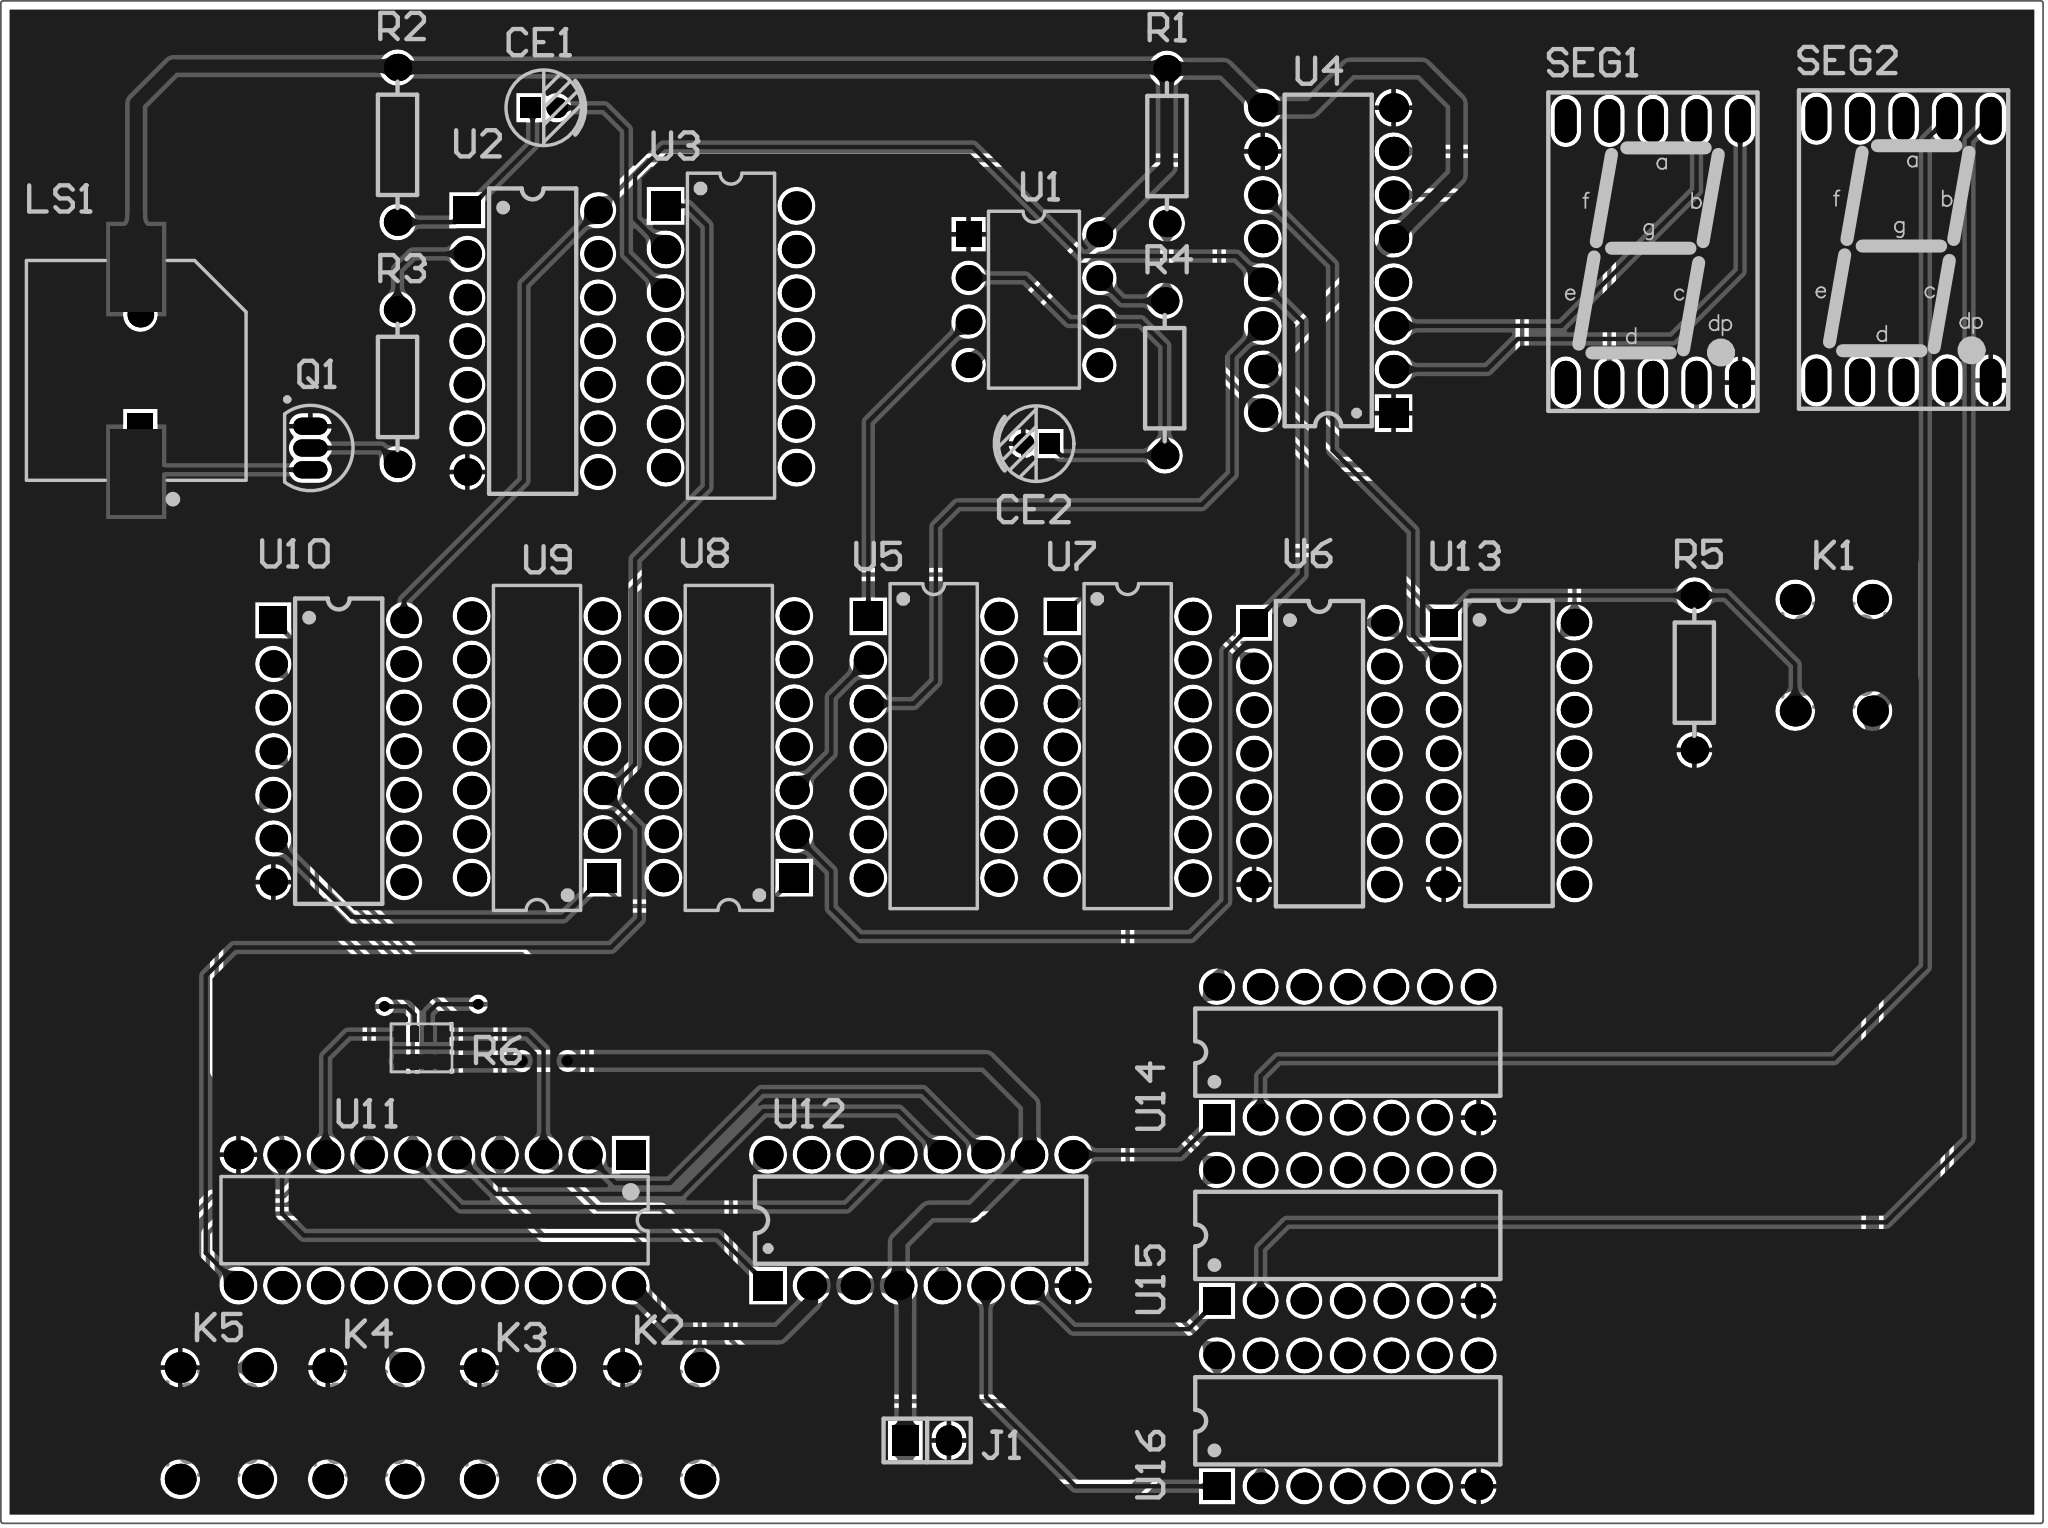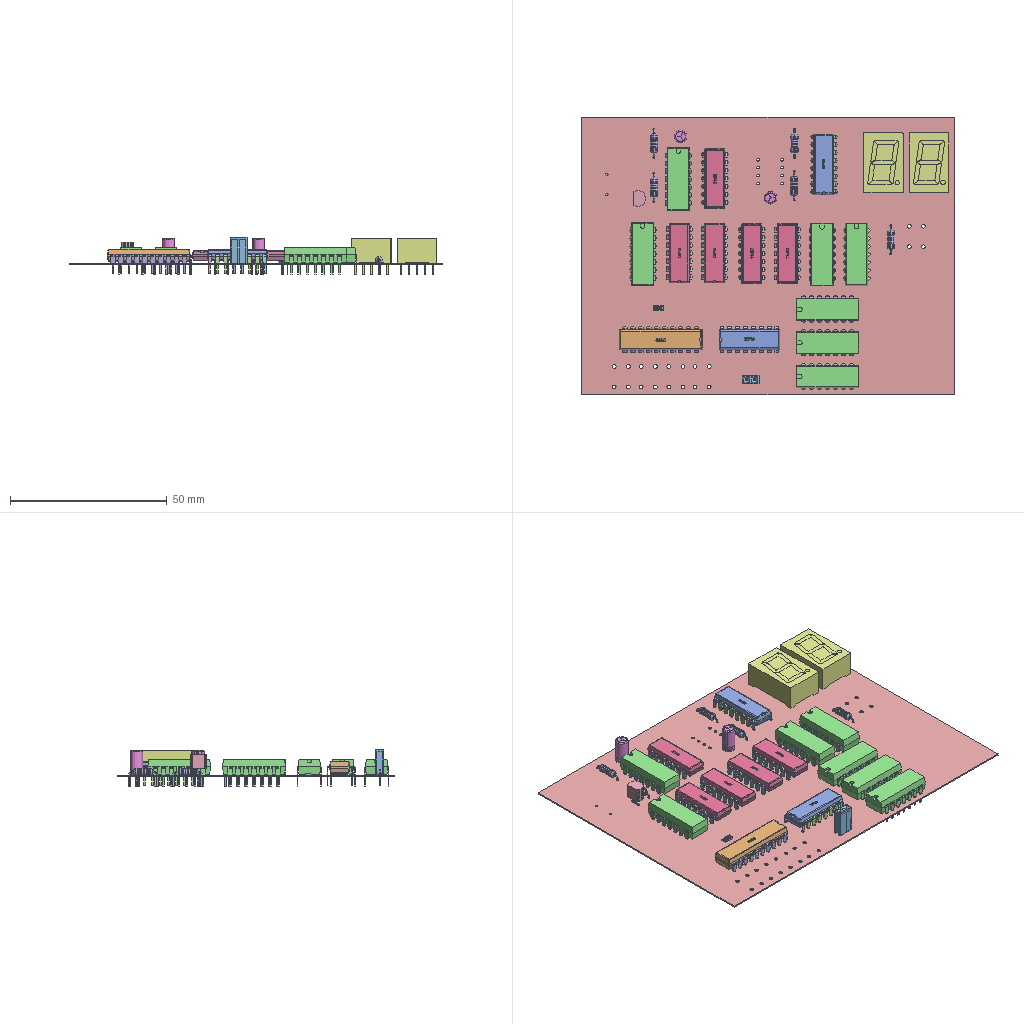Circuit board layout | Altium Designer | box 119 x 88.6 x 12.1 mm
Layer stack:
# Altium Designer layer stack of  (unit mm; dielectric type: 0 none, 1 core, 2 prepreg, 3 surface material)
index,name,kind,layer,copper_thickness_mm,dielectric_type,dielectric_thickness_mm,dielectric_material,dielectric_constant
0,Top Paste,other,,,,,,
1,Top Overlay,other,,,,,,
2,Top Solder,dielectric,,,3,0.0102,Solder Resist,3.5
3,Top Layer,copper,Top Layer,0.0356,,,,
4,Dielectric 1,dielectric,,,0,0.32,FR-4,4.8
5,Bottom Layer,copper,Bottom Layer,0.0356,,,,
6,Bottom Solder,dielectric,,,3,0.0102,Solder Resist,3.5
7,Bottom Overlay,other,,,,,,
8,Bottom Paste,other,,,,,,
# drill layer pairs: low layer,high layer
drill_pair,Top Layer,Bottom Layer
Part placement:
Designator,Comment,Layer,Footprint,Center-X(mm),Center-Y(mm),Rotation
U12,74LS148,TopLayer,DIP16,80.772,33.909,90
U11,DM74LS373N,TopLayer,DIP20,52.451,33.909,270
U10,74LS21,TopLayer,DIP14,46.863,61.214,0
U9,74LS32,TopLayer,DIP14,58.42,61.468,180
U8,74LS08,TopLayer,DIP14,69.596,61.468,180
U7,74LS32,TopLayer,DIP14,92.837,61.445,0
U5,74LS08,TopLayer,DIP14,81.534,61.445,360
U4,74LS190,TopLayer,DIP16,104.521,89.789,180
U3,74LS08,TopLayer,DIP14,69.723,85.344,0
U2,74F04N,TopLayer,DIP14,58.166,85.09,0
U1,LM555,TopLayer,J08A,87.376,87.503,270
SEG2,0.56IN-1-K,TopLayer,0.56IN-1P,138.049,90.424,0
SEG1,0.56IN-1-K,TopLayer,0.56IN-1P,123.444,90.297,360
R6,103,TopLayer,RCA-8P4R-0603,51.689,43.942,180
R5,10K,TopLayer,RS_1/4W,125.857,65.786,90
R4,68K,TopLayer,RS_1/4W,94.996,82.931,90
R3,10K,TopLayer,RS_1/4W,50.292,82.423,90
R2,47K,TopLayer,RS_1/4W,50.292,96.52,90
R1,1K,TopLayer,RS_1/4W,95.123,96.448,90
Q1,2N3904,TopLayer,TO-92A,45.212,78.867,180
LS1,Buzzer,TopLayer,ABSM-1574,35.186,83.387,90
K5,KEY,TopLayer,四脚轻触开关,39.878,22.075,90
K4,KEY,TopLayer,四脚轻触开关,48.478,22.075,90
K3,KEY,TopLayer,四脚轻触开关,57.313,22.075,90
K2,KEY,TopLayer,四脚轻触开关,65.659,22.075,90
K1,KEY,TopLayer,四脚轻触开关,133.985,66.802,270
J1,Female HDR1X2,TopLayer,Fe-HDR1X2/2.54-S,81.153,21.082,360
CE2,10uF,TopLayer,CAP_1.5*4*8,87.503,79.121,180
CE1,10uF,TopLayer,CAP_1.5*4*8,58.813,98.679,360
U6,SN74F04N,TopLayer,DIP14,104.013,61.07,360
U13,SN74F04N,TopLayer,DIP14,115.062,61.087,0
U14,SN74F04N,TopLayer,DIP14,105.664,43.688,90
U15,SN74F04N,TopLayer,DIP14,105.664,33.02,90
U16,SN74F04N,TopLayer,DIP14,105.664,22.225,90
Pad and via stacks:
# Altium Designer via and pad stacks of  (unit mm). Each distinct definition once, with the count of objects using it.
# via: kind,start_layer,end_layer,hole_mm,diameter_mm,mode(0 simple;1 top-mid-bottom;2 full stack),diameter_per_layer,count,example_net
# pad: kind,layer,hole_mm,hole_type(0 round;1 square;2 slot),plating,top_size,top_shape(1 round;2 rect;3 octagon;9 rounded rect),mid_size,bottom_size,mode,footprint,size_per_layer,count,example
pad,Multi-Layer,0.7,0,plated,1.5x1.5,2,1.5x1.5,1.5x1.5,0,ABSM-1574,,1,LS1.1A
pad,Multi-Layer,0.7,0,plated,1.5x1.5,1,1.5x1.5,1.5x1.5,0,ABSM-1574,,1,LS1.2A
pad,Multi-Layer,0.6,0,plated,1.6x1.6,1,1.6x1.6,1.6x1.6,0,RS 1/4W,,10,R1.2
pad,Multi-Layer,0.9,0,plated,1.5x1.5,2,1.5x1.5,1.5x1.5,0,J08A,,1,U1.1
pad,Multi-Layer,0.9,0,plated,1.5x1.5,1,1.5x1.5,1.5x1.5,0,J08A,,7,U1.2
pad,Multi-Layer,0.8,0,plated,1.7x1.7,2,1.7x1.7,1.7x1.7,0,DIP14,,5,U3.1
pad,Multi-Layer,0.8,0,plated,1.7x1.7,1,1.7x1.7,1.7x1.7,0,DIP14,,65,U3.2
pad,Multi-Layer,0.8128,0,plated,1.6x1.6,1,1.6x1.6,1.6x1.6,0,DIP14,,91,U2.14
pad,Multi-Layer,0.8128,0,plated,1.6x1.6,2,1.6x1.6,1.6x1.6,0,DIP14,,7,U2.1
pad,Multi-Layer,0.8,0,plated,1.7x1.7,1,1.7x1.7,1.7x1.7,0,DIP16,,30,U4.16
pad,Multi-Layer,0.8,0,plated,1.7x1.7,2,1.7x1.7,1.7x1.7,0,DIP16,,2,U4.1
pad,Multi-Layer,0.6,0,plated,1.2x1.2,1,1.2x1.2,1.2x1.2,0,CAP 1.5*4*8,,2,CE1.2
pad,Multi-Layer,0.6,0,plated,1.2x1.2,2,1.2x1.2,1.2x1.2,0,CAP 1.5*4*8,,2,CE1.1
pad,Multi-Layer,0.9,0,plated,2x1,1,2x1,2x1,0,TO-92A,,3,Q1.3
pad,Multi-Layer,0.85,0,plated,2.54x1.27,1,2.54x1.27,2.54x1.27,0,0.56IN-1P,,20,SEG1.10
pad,Multi-Layer,0.8128,0,plated,1.524x1.778,2,1.524x1.778,1.524x1.778,0,Fe-HDR1X2/2.54-S,,1,J1.1
pad,Multi-Layer,0.8128,0,plated,1.524x1.778,1,1.524x1.778,1.524x1.778,0,Fe-HDR1X2/2.54-S,,1,J1.2
pad,Multi-Layer,0.8,0,plated,1.7x1.7,1,1.7x1.7,1.7x1.7,0,DIP20,,19,U11.11
pad,Multi-Layer,0.8,0,plated,1.7x1.7,2,1.7x1.7,1.7x1.7,0,DIP20,,1,U11.1
pad,Multi-Layer,1.2,0,plated,1.8x1.8,1,1.8x1.8,1.8x1.8,0,\u00CB\u00C4\u00BD\u00C5\u00C7\u00E1\u00B4\u00A5\u00BF\u00AA\u00B9\u00D8,,20,K1.4
pad,Top Layer,0,0,plated,3x5,2,3x5,3x5,0,ABSM-1574,,2,LS1.1
pad,Top Layer,0,0,plated,0.65x0.9,2,0.65x0.9,0.65x0.9,0,RCA-8P4R-0603,,4,R6.8
pad,Top Layer,0,0,plated,0.5x0.9,2,0.5x0.9,0.5x0.9,0,RCA-8P4R-0603,,4,R6.7
via,Top Layer,Bottom Layer,0.3048,0.6096,0,,4,NetK3_3
Copper pours:
name,layer,net,type(0 solid;1 hatched;2 none)
D,Top Layer,GND,0
D,Bottom Layer,GND,0
Design rules, without the lines most boards share:
# Altium Designer design rules of  (exported by Altium Designer, unit mm)
# columns: name | kind | enabled | priority | scope1 | scope2 | descriptor | typed fields (field=value)
SilkToSilkClearance | 55 | enabled | 1 | All | All | Silk to Silk (Clearance=0mil) (All),(All) |
SilkToSolderMaskClearance | 54 | enabled | 1 | IsPad | All | Silk To Solder Mask (Clearance=0mil) (IsPad),(All) |
MinimumSolderMaskSliver | 53 | enabled | 1 | All | All | Minimum Solder Mask Sliver (Gap=0mil) (All),(All) |
HoleToHoleClearance | 52 | enabled | 1 | All | All | Hole To Hole Clearance (Gap=10mil) (All),(All) | gap=0.254
DiffPairsRouting | 51 | enabled | 1 | All | All | Differential Pairs Uncoupled Length using the Gap Constraints (Min=10mil) (Max=10mil) (Prefered=10mil)  and Width Constraints (Min=15mil) (Max=15mil) (Prefered=15mil) (All) |
HoleSize | 42 | enabled | 1 | All | All | Hole Size Constraint (Min=1mil) (Max=4444mil) (All) |
SolderMaskExpansion | 13 | enabled | 1 | All | All | Solder Mask Expansion (Expansion =4mil) (All) | expansion=0.1016
PasteMaskExpansion | 14 | enabled | 1 | All | All | Paste Mask Expansion (Expansion =0mil) (All) | expansion=0
RoutingVias | 11 | enabled | 1 | All | All | Routing Via (MinHoleWidth=28mil) (MaxHoleWidth=28mil) (PreferredHoleWidth=28mil) (MinWidth=50mil) (MaxWidth=50mil) (PreferedWidth=50mil) (All) | via_min_hole=0.7112 via_max_hole=0.7112 via_preferred_diameter=1.27 via_preferred_hole=0.7112
Width | 2 | enabled | 1 | All | All | Width Constraint (Min=10mil) (Max=500mil) (Preferred=10mil) (All) |
PolygonConnect | 20 | enabled | 1 | All | All | Polygon Connect Rule(Relief Connect )(Conductor Width=10mil) (Relief Angle=90 Angle) (Entries=4) (Air Gap Width=10mil) (All),(All) | connect_style(0=relief,1=direct,2=none)=0 relief_conductor_width=0.254 relief_entries=4
PlaneConnect | 6 | enabled | 1 | All | All | Power Plane Connect Rule(Relief Connect )(Expansion=20mil) (Conductor Width=10mil) (Air Gap=10mil) (Entries=4) (All) | relief_conductor_width=0.254 relief_entries=4 relief_expansion=0.508
Clearance | 0 | enabled | 1 | All | All | Clearance Constraint (Gap=10mil) (All),(All) | gap=0.254
Classes set for this board:
# Altium Designer classes of  (member kind: 0 net, 1 component, 2 from-to, 3 pad, 4 layer, 5 differential pair, 6 design channel, 7 polygon, 8 structure, 9 xSignal)
# columns: class name | member kind | superclass | members
Sheet1 | 1 | no | CE1; CE2; J1; K1; K2; K3; K4; K5; LS1; Q1; R1; R2; R3; R4; R5; R6; SEG1; SEG2; U1; U2; U3; U4; U5; U12; U13; U14; U15; U16; U12; U8; U7; U10; U11; U9; U6;